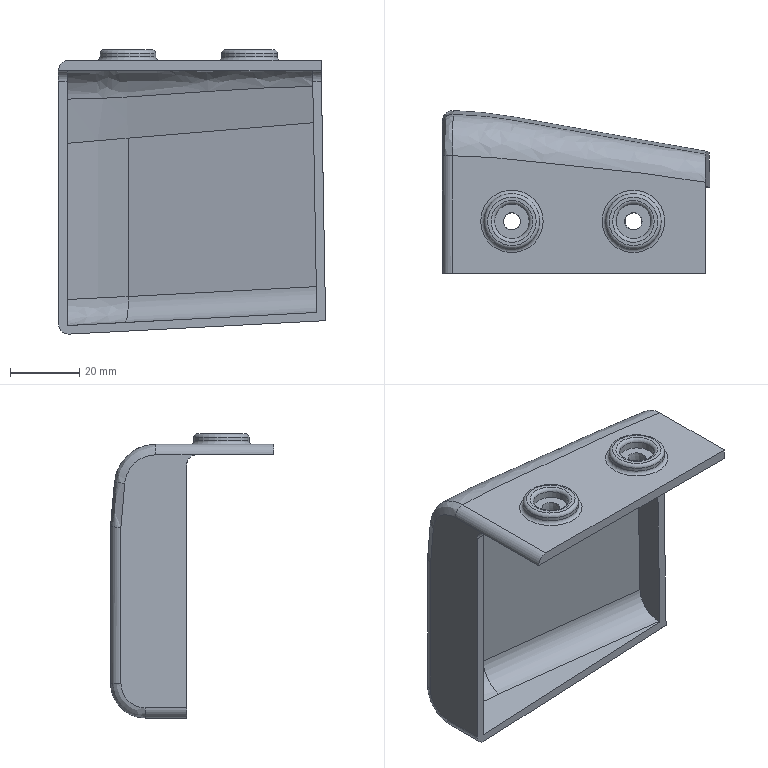Part | STEP file | HGL | 1 solid | 48 faces | box 76.93 x 46.944 x 81.839 mm | volume 29643 mm3 | plane 18 | cylinder 13 | spline 9 | torus 6 | cone 2 | commonest cylinder face diameters 6 x5 10 x2 16 x2 15 x1 20 x1 235 x1